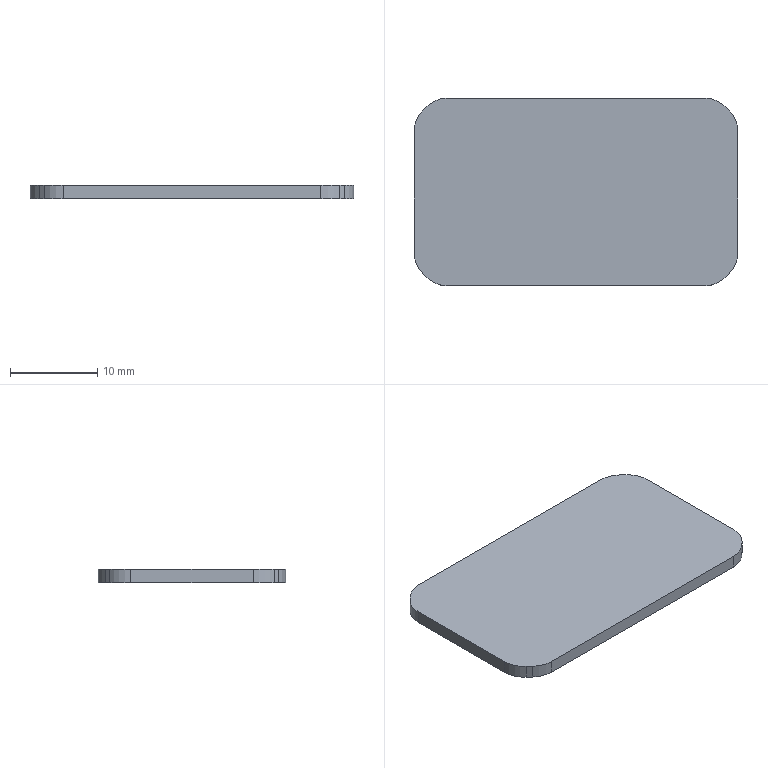Part | SolidWorks | features BaseBody 1 | 1 solid | 18 faces | box 37.1 x 21.5 x 1.5 mm | volume 1176 mm3 | plane 10 | cylinder 8 | commonest cylinder face diameters 6.5 x8
STEP:
#1=CARTESIAN_POINT('',(-18.55,7.,1.5));
#2=VERTEX_POINT('',#1);
#3=CARTESIAN_POINT('',(-18.55,-7.,1.5));
#4=VERTEX_POINT('',#3);
#5=CARTESIAN_POINT('',(-18.55,7.,1.5));
#6=DIRECTION('',(0.,-1.,0.));
#7=VECTOR('',#6,1000.);
#8=LINE('',#5,#7);
#9=EDGE_CURVE('',#2,#4,#8,.T.);
#10=ORIENTED_EDGE('',*,*,#9,.T.);
#11=CARTESIAN_POINT('',(-17.486,-9.405,1.5));
#12=VERTEX_POINT('',#11);
#13=CARTESIAN_POINT('',(-15.3,-7.,1.5));
#14=DIRECTION('',(0.,0.,1.));
#15=DIRECTION('',(-1.,0.,0.));
#16=AXIS2_PLACEMENT_3D('',#13,#14,#15);
#17=CIRCLE('',#16,3.25);
#18=EDGE_CURVE('',#4,#12,#17,.T.);
#19=ORIENTED_EDGE('',*,*,#18,.T.);
#20=CARTESIAN_POINT('',(-16.936,-9.905,1.5));
#21=VERTEX_POINT('',#20);
#22=CARTESIAN_POINT('',(-17.486,-9.405,1.5));
#23=DIRECTION('',(0.7399,-0.6727,0.));
#24=VECTOR('',#23,1000.);
#25=LINE('',#22,#24);
#26=EDGE_CURVE('',#12,#21,#25,.T.);
#27=ORIENTED_EDGE('',*,*,#26,.T.);
#28=CARTESIAN_POINT('',(-14.75,-10.75,1.5));
#29=VERTEX_POINT('',#28);
#30=CARTESIAN_POINT('',(-14.75,-7.5,1.5));
#31=DIRECTION('',(0.,0.,1.));
#32=DIRECTION('',(-0.6727,-0.7399,0.));
#33=AXIS2_PLACEMENT_3D('',#30,#31,#32);
#34=CIRCLE('',#33,3.25);
#35=EDGE_CURVE('',#21,#29,#34,.T.);
#36=ORIENTED_EDGE('',*,*,#35,.T.);
#37=CARTESIAN_POINT('',(14.75,-10.75,1.5));
#38=VERTEX_POINT('',#37);
#39=CARTESIAN_POINT('',(-14.75,-10.75,1.5));
#40=DIRECTION('',(1.,0.,0.));
#41=VECTOR('',#40,1000.);
#42=LINE('',#39,#41);
#43=EDGE_CURVE('',#29,#38,#42,.T.);
#44=ORIENTED_EDGE('',*,*,#43,.T.);
#45=CARTESIAN_POINT('',(16.936,-9.905,1.5));
#46=VERTEX_POINT('',#45);
#47=CARTESIAN_POINT('',(14.75,-7.5,1.5));
#48=DIRECTION('',(0.,0.,1.));
#49=DIRECTION('',(0.,-1.,0.));
#50=AXIS2_PLACEMENT_3D('',#47,#48,#49);
#51=CIRCLE('',#50,3.25);
#52=EDGE_CURVE('',#38,#46,#51,.T.);
#53=ORIENTED_EDGE('',*,*,#52,.T.);
#54=CARTESIAN_POINT('',(17.486,-9.405,1.5));
#55=VERTEX_POINT('',#54);
#56=CARTESIAN_POINT('',(16.936,-9.905,1.5));
#57=DIRECTION('',(0.7399,0.6727,0.));
#58=VECTOR('',#57,1000.);
#59=LINE('',#56,#58);
#60=EDGE_CURVE('',#46,#55,#59,.T.);
#61=ORIENTED_EDGE('',*,*,#60,.T.);
#62=CARTESIAN_POINT('',(18.55,-7.,1.5));
#63=VERTEX_POINT('',#62);
#64=CARTESIAN_POINT('',(15.3,-7.,1.5));
#65=DIRECTION('',(0.,0.,1.));
#66=DIRECTION('',(0.6727,-0.7399,0.));
#67=AXIS2_PLACEMENT_3D('',#64,#65,#66);
#68=CIRCLE('',#67,3.25);
#69=EDGE_CURVE('',#55,#63,#68,.T.);
#70=ORIENTED_EDGE('',*,*,#69,.T.);
#71=CARTESIAN_POINT('',(18.55,7.,1.5));
#72=VERTEX_POINT('',#71);
#73=CARTESIAN_POINT('',(18.55,-7.,1.5));
#74=DIRECTION('',(0.,1.,0.));
#75=VECTOR('',#74,1000.);
#76=LINE('',#73,#75);
#77=EDGE_CURVE('',#63,#72,#76,.T.);
#78=ORIENTED_EDGE('',*,*,#77,.T.);
#79=CARTESIAN_POINT('',(17.486,9.405,1.5));
#80=VERTEX_POINT('',#79);
#81=CARTESIAN_POINT('',(15.3,7.,1.5));
#82=DIRECTION('',(0.,0.,1.));
#83=DIRECTION('',(1.,0.,0.));
#84=AXIS2_PLACEMENT_3D('',#81,#82,#83);
#85=CIRCLE('',#84,3.25);
#86=EDGE_CURVE('',#72,#80,#85,.T.);
#87=ORIENTED_EDGE('',*,*,#86,.T.);
#88=CARTESIAN_POINT('',(16.936,9.905,1.5));
#89=VERTEX_POINT('',#88);
#90=CARTESIAN_POINT('',(17.486,9.405,1.5));
#91=DIRECTION('',(-0.7399,0.6727,0.));
#92=VECTOR('',#91,1000.);
#93=LINE('',#90,#92);
#94=EDGE_CURVE('',#80,#89,#93,.T.);
#95=ORIENTED_EDGE('',*,*,#94,.T.);
#96=CARTESIAN_POINT('',(14.75,10.75,1.5));
#97=VERTEX_POINT('',#96);
#98=CARTESIAN_POINT('',(14.75,7.5,1.5));
#99=DIRECTION('',(0.,0.,1.));
#100=DIRECTION('',(0.6727,0.7399,0.));
#101=AXIS2_PLACEMENT_3D('',#98,#99,#100);
#102=CIRCLE('',#101,3.25);
#103=EDGE_CURVE('',#89,#97,#102,.T.);
#104=ORIENTED_EDGE('',*,*,#103,.T.);
#105=CARTESIAN_POINT('',(-14.75,10.75,1.5));
#106=VERTEX_POINT('',#105);
#107=CARTESIAN_POINT('',(14.75,10.75,1.5));
#108=DIRECTION('',(-1.,0.,0.));
#109=VECTOR('',#108,1000.);
#110=LINE('',#107,#109);
#111=EDGE_CURVE('',#97,#106,#110,.T.);
#112=ORIENTED_EDGE('',*,*,#111,.T.);
#113=CARTESIAN_POINT('',(-16.936,9.905,1.5));
#114=VERTEX_POINT('',#113);
#115=CARTESIAN_POINT('',(-14.75,7.5,1.5));
#116=DIRECTION('',(0.,0.,1.));
#117=DIRECTION('',(0.,1.,0.));
#118=AXIS2_PLACEMENT_3D('',#115,#116,#117);
#119=CIRCLE('',#118,3.25);
#120=EDGE_CURVE('',#106,#114,#119,.T.);
#121=ORIENTED_EDGE('',*,*,#120,.T.);
#122=CARTESIAN_POINT('',(-17.486,9.405,1.5));
#123=VERTEX_POINT('',#122);
#124=CARTESIAN_POINT('',(-16.936,9.905,1.5));
#125=DIRECTION('',(-0.7399,-0.6727,0.));
#126=VECTOR('',#125,1000.);
#127=LINE('',#124,#126);
#128=EDGE_CURVE('',#114,#123,#127,.T.);
#129=ORIENTED_EDGE('',*,*,#128,.T.);
#130=CARTESIAN_POINT('',(-15.3,7.,1.5));
#131=DIRECTION('',(0.,0.,1.));
#132=DIRECTION('',(-0.6727,0.7399,0.));
#133=AXIS2_PLACEMENT_3D('',#130,#131,#132);
#134=CIRCLE('',#133,3.25);
#135=EDGE_CURVE('',#123,#2,#134,.T.);
#136=ORIENTED_EDGE('',*,*,#135,.T.);
#137=EDGE_LOOP('',(#10,#19,#27,#36,#44,#53,#61,#70,#78,#87,#95,#104,#112,#121,#129,#136));
#138=FACE_OUTER_BOUND('',#137,.T.);
#139=CARTESIAN_POINT('',(0.,0.,1.5));
#140=DIRECTION('',(0.,0.,1.));
#141=DIRECTION('',(1.,0.,0.));
#142=AXIS2_PLACEMENT_3D('',#139,#140,#141);
#143=PLANE('',#142);
#144=ADVANCED_FACE('',(#138),#143,.T.);
#145=CARTESIAN_POINT('',(-18.55,-7.,0.));
#146=VERTEX_POINT('',#145);
#147=CARTESIAN_POINT('',(-18.55,-7.,0.));
#148=DIRECTION('',(0.,0.,1.));
#149=VECTOR('',#148,1000.);
#150=LINE('',#147,#149);
#151=EDGE_CURVE('',#146,#4,#150,.T.);
#152=ORIENTED_EDGE('',*,*,#151,.T.);
#153=ORIENTED_EDGE('',*,*,#9,.F.);
#154=CARTESIAN_POINT('',(-18.55,7.,0.));
#155=VERTEX_POINT('',#154);
#156=CARTESIAN_POINT('',(-18.55,7.,0.));
#157=DIRECTION('',(0.,0.,1.));
#158=VECTOR('',#157,1000.);
#159=LINE('',#156,#158);
#160=EDGE_CURVE('',#155,#2,#159,.T.);
#161=ORIENTED_EDGE('',*,*,#160,.F.);
#162=CARTESIAN_POINT('',(-18.55,7.,0.));
#163=DIRECTION('',(0.,-1.,0.));
#164=VECTOR('',#163,1000.);
#165=LINE('',#162,#164);
#166=EDGE_CURVE('',#155,#146,#165,.T.);
#167=ORIENTED_EDGE('',*,*,#166,.T.);
#168=EDGE_LOOP('',(#152,#153,#161,#167));
#169=FACE_OUTER_BOUND('',#168,.T.);
#170=CARTESIAN_POINT('',(-18.55,7.,0.));
#171=DIRECTION('',(-1.,0.,0.));
#172=DIRECTION('',(0.,0.,1.));
#173=AXIS2_PLACEMENT_3D('',#170,#171,#172);
#174=PLANE('',#173);
#175=ADVANCED_FACE('',(#169),#174,.T.);
#176=CARTESIAN_POINT('',(-17.486,-9.405,0.));
#177=VERTEX_POINT('',#176);
#178=CARTESIAN_POINT('',(-17.486,-9.405,0.));
#179=DIRECTION('',(0.,0.,1.));
#180=VECTOR('',#179,1000.);
#181=LINE('',#178,#180);
#182=EDGE_CURVE('',#177,#12,#181,.T.);
#183=ORIENTED_EDGE('',*,*,#182,.T.);
#184=ORIENTED_EDGE('',*,*,#18,.F.);
#185=ORIENTED_EDGE('',*,*,#151,.F.);
#186=CARTESIAN_POINT('',(-15.3,-7.,0.));
#187=DIRECTION('',(0.,0.,1.));
#188=DIRECTION('',(-1.,0.,0.));
#189=AXIS2_PLACEMENT_3D('',#186,#187,#188);
#190=CIRCLE('',#189,3.25);
#191=EDGE_CURVE('',#146,#177,#190,.T.);
#192=ORIENTED_EDGE('',*,*,#191,.T.);
#193=EDGE_LOOP('',(#183,#184,#185,#192));
#194=FACE_OUTER_BOUND('',#193,.T.);
#195=CARTESIAN_POINT('',(-15.3,-7.,0.));
#196=DIRECTION('',(0.,0.,1.));
#197=DIRECTION('',(1.,0.,0.));
#198=AXIS2_PLACEMENT_3D('',#195,#196,#197);
#199=CYLINDRICAL_SURFACE('',#198,3.25);
#200=ADVANCED_FACE('',(#194),#199,.T.);
#201=CARTESIAN_POINT('',(-16.936,-9.905,0.));
#202=VERTEX_POINT('',#201);
#203=CARTESIAN_POINT('',(-16.936,-9.905,0.));
#204=DIRECTION('',(0.,0.,1.));
#205=VECTOR('',#204,1000.);
#206=LINE('',#203,#205);
#207=EDGE_CURVE('',#202,#21,#206,.T.);
#208=ORIENTED_EDGE('',*,*,#207,.T.);
#209=ORIENTED_EDGE('',*,*,#26,.F.);
#210=ORIENTED_EDGE('',*,*,#182,.F.);
#211=CARTESIAN_POINT('',(-17.486,-9.405,0.));
#212=DIRECTION('',(0.7399,-0.6727,0.));
#213=VECTOR('',#212,1000.);
#214=LINE('',#211,#213);
#215=EDGE_CURVE('',#177,#202,#214,.T.);
#216=ORIENTED_EDGE('',*,*,#215,.T.);
#217=EDGE_LOOP('',(#208,#209,#210,#216));
#218=FACE_OUTER_BOUND('',#217,.T.);
#219=CARTESIAN_POINT('',(-17.486,-9.405,0.));
#220=DIRECTION('',(-0.6727,-0.7399,0.));
#221=DIRECTION('',(-0.7399,0.6727,0.));
#222=AXIS2_PLACEMENT_3D('',#219,#220,#221);
#223=PLANE('',#222);
#224=ADVANCED_FACE('',(#218),#223,.T.);
#225=CARTESIAN_POINT('',(-14.75,-10.75,0.));
#226=VERTEX_POINT('',#225);
#227=CARTESIAN_POINT('',(-14.75,-10.75,0.));
#228=DIRECTION('',(0.,0.,1.));
#229=VECTOR('',#228,1000.);
#230=LINE('',#227,#229);
#231=EDGE_CURVE('',#226,#29,#230,.T.);
#232=ORIENTED_EDGE('',*,*,#231,.T.);
#233=ORIENTED_EDGE('',*,*,#35,.F.);
#234=ORIENTED_EDGE('',*,*,#207,.F.);
#235=CARTESIAN_POINT('',(-14.75,-7.5,0.));
#236=DIRECTION('',(0.,0.,1.));
#237=DIRECTION('',(-0.6727,-0.7399,0.));
#238=AXIS2_PLACEMENT_3D('',#235,#236,#237);
#239=CIRCLE('',#238,3.25);
#240=EDGE_CURVE('',#202,#226,#239,.T.);
#241=ORIENTED_EDGE('',*,*,#240,.T.);
#242=EDGE_LOOP('',(#232,#233,#234,#241));
#243=FACE_OUTER_BOUND('',#242,.T.);
#244=CARTESIAN_POINT('',(-14.75,-7.5,0.));
#245=DIRECTION('',(0.,0.,1.));
#246=DIRECTION('',(1.,0.,0.));
#247=AXIS2_PLACEMENT_3D('',#244,#245,#246);
#248=CYLINDRICAL_SURFACE('',#247,3.25);
#249=ADVANCED_FACE('',(#243),#248,.T.);
#250=CARTESIAN_POINT('',(14.75,-10.75,0.));
#251=VERTEX_POINT('',#250);
#252=CARTESIAN_POINT('',(14.75,-10.75,0.));
#253=DIRECTION('',(0.,0.,1.));
#254=VECTOR('',#253,1000.);
#255=LINE('',#252,#254);
#256=EDGE_CURVE('',#251,#38,#255,.T.);
#257=ORIENTED_EDGE('',*,*,#256,.T.);
#258=ORIENTED_EDGE('',*,*,#43,.F.);
#259=ORIENTED_EDGE('',*,*,#231,.F.);
#260=CARTESIAN_POINT('',(-14.75,-10.75,0.));
#261=DIRECTION('',(1.,0.,0.));
#262=VECTOR('',#261,1000.);
#263=LINE('',#260,#262);
#264=EDGE_CURVE('',#226,#251,#263,.T.);
#265=ORIENTED_EDGE('',*,*,#264,.T.);
#266=EDGE_LOOP('',(#257,#258,#259,#265));
#267=FACE_OUTER_BOUND('',#266,.T.);
#268=CARTESIAN_POINT('',(-14.75,-10.75,0.));
#269=DIRECTION('',(0.,-1.,0.));
#270=DIRECTION('',(0.,0.,-1.));
#271=AXIS2_PLACEMENT_3D('',#268,#269,#270);
#272=PLANE('',#271);
#273=ADVANCED_FACE('',(#267),#272,.T.);
#274=CARTESIAN_POINT('',(16.936,-9.905,0.));
#275=VERTEX_POINT('',#274);
#276=CARTESIAN_POINT('',(16.936,-9.905,0.));
#277=DIRECTION('',(0.,0.,1.));
#278=VECTOR('',#277,1000.);
#279=LINE('',#276,#278);
#280=EDGE_CURVE('',#275,#46,#279,.T.);
#281=ORIENTED_EDGE('',*,*,#280,.T.);
#282=ORIENTED_EDGE('',*,*,#52,.F.);
#283=ORIENTED_EDGE('',*,*,#256,.F.);
#284=CARTESIAN_POINT('',(14.75,-7.5,0.));
#285=DIRECTION('',(0.,0.,1.));
#286=DIRECTION('',(0.,-1.,0.));
#287=AXIS2_PLACEMENT_3D('',#284,#285,#286);
#288=CIRCLE('',#287,3.25);
#289=EDGE_CURVE('',#251,#275,#288,.T.);
#290=ORIENTED_EDGE('',*,*,#289,.T.);
#291=EDGE_LOOP('',(#281,#282,#283,#290));
#292=FACE_OUTER_BOUND('',#291,.T.);
#293=CARTESIAN_POINT('',(14.75,-7.5,0.));
#294=DIRECTION('',(0.,0.,1.));
#295=DIRECTION('',(1.,0.,0.));
#296=AXIS2_PLACEMENT_3D('',#293,#294,#295);
#297=CYLINDRICAL_SURFACE('',#296,3.25);
#298=ADVANCED_FACE('',(#292),#297,.T.);
#299=CARTESIAN_POINT('',(17.486,-9.405,0.));
#300=VERTEX_POINT('',#299);
#301=CARTESIAN_POINT('',(17.486,-9.405,0.));
#302=DIRECTION('',(0.,0.,1.));
#303=VECTOR('',#302,1000.);
#304=LINE('',#301,#303);
#305=EDGE_CURVE('',#300,#55,#304,.T.);
#306=ORIENTED_EDGE('',*,*,#305,.T.);
#307=ORIENTED_EDGE('',*,*,#60,.F.);
#308=ORIENTED_EDGE('',*,*,#280,.F.);
#309=CARTESIAN_POINT('',(16.936,-9.905,0.));
#310=DIRECTION('',(0.7399,0.6727,0.));
#311=VECTOR('',#310,1000.);
#312=LINE('',#309,#311);
#313=EDGE_CURVE('',#275,#300,#312,.T.);
#314=ORIENTED_EDGE('',*,*,#313,.T.);
#315=EDGE_LOOP('',(#306,#307,#308,#314));
#316=FACE_OUTER_BOUND('',#315,.T.);
#317=CARTESIAN_POINT('',(16.936,-9.905,0.));
#318=DIRECTION('',(0.6727,-0.7399,0.));
#319=DIRECTION('',(0.,0.,-1.));
#320=AXIS2_PLACEMENT_3D('',#317,#318,#319);
#321=PLANE('',#320);
#322=ADVANCED_FACE('',(#316),#321,.T.);
#323=CARTESIAN_POINT('',(18.55,-7.,0.));
#324=VERTEX_POINT('',#323);
#325=CARTESIAN_POINT('',(18.55,-7.,0.));
#326=DIRECTION('',(0.,0.,1.));
#327=VECTOR('',#326,1000.);
#328=LINE('',#325,#327);
#329=EDGE_CURVE('',#324,#63,#328,.T.);
#330=ORIENTED_EDGE('',*,*,#329,.T.);
#331=ORIENTED_EDGE('',*,*,#69,.F.);
#332=ORIENTED_EDGE('',*,*,#305,.F.);
#333=CARTESIAN_POINT('',(15.3,-7.,0.));
#334=DIRECTION('',(0.,0.,1.));
#335=DIRECTION('',(0.6727,-0.7399,0.));
#336=AXIS2_PLACEMENT_3D('',#333,#334,#335);
#337=CIRCLE('',#336,3.25);
#338=EDGE_CURVE('',#300,#324,#337,.T.);
#339=ORIENTED_EDGE('',*,*,#338,.T.);
#340=EDGE_LOOP('',(#330,#331,#332,#339));
#341=FACE_OUTER_BOUND('',#340,.T.);
#342=CARTESIAN_POINT('',(15.3,-7.,0.));
#343=DIRECTION('',(0.,0.,1.));
#344=DIRECTION('',(1.,0.,0.));
#345=AXIS2_PLACEMENT_3D('',#342,#343,#344);
#346=CYLINDRICAL_SURFACE('',#345,3.25);
#347=ADVANCED_FACE('',(#341),#346,.T.);
#348=CARTESIAN_POINT('',(18.55,7.,0.));
#349=VERTEX_POINT('',#348);
#350=CARTESIAN_POINT('',(18.55,7.,0.));
#351=DIRECTION('',(0.,0.,1.));
#352=VECTOR('',#351,1000.);
#353=LINE('',#350,#352);
#354=EDGE_CURVE('',#349,#72,#353,.T.);
#355=ORIENTED_EDGE('',*,*,#354,.T.);
#356=ORIENTED_EDGE('',*,*,#77,.F.);
#357=ORIENTED_EDGE('',*,*,#329,.F.);
#358=CARTESIAN_POINT('',(18.55,-7.,0.));
#359=DIRECTION('',(0.,1.,0.));
#360=VECTOR('',#359,1000.);
#361=LINE('',#358,#360);
#362=EDGE_CURVE('',#324,#349,#361,.T.);
#363=ORIENTED_EDGE('',*,*,#362,.T.);
#364=EDGE_LOOP('',(#355,#356,#357,#363));
#365=FACE_OUTER_BOUND('',#364,.T.);
#366=CARTESIAN_POINT('',(18.55,-7.,0.));
#367=DIRECTION('',(1.,0.,0.));
#368=DIRECTION('',(0.,1.,0.));
#369=AXIS2_PLACEMENT_3D('',#366,#367,#368);
#370=PLANE('',#369);
#371=ADVANCED_FACE('',(#365),#370,.T.);
#372=CARTESIAN_POINT('',(17.486,9.405,0.));
#373=VERTEX_POINT('',#372);
#374=CARTESIAN_POINT('',(17.486,9.405,0.));
#375=DIRECTION('',(0.,0.,1.));
#376=VECTOR('',#375,1000.);
#377=LINE('',#374,#376);
#378=EDGE_CURVE('',#373,#80,#377,.T.);
#379=ORIENTED_EDGE('',*,*,#378,.T.);
#380=ORIENTED_EDGE('',*,*,#86,.F.);
#381=ORIENTED_EDGE('',*,*,#354,.F.);
#382=CARTESIAN_POINT('',(15.3,7.,0.));
#383=DIRECTION('',(0.,0.,1.));
#384=DIRECTION('',(1.,0.,0.));
#385=AXIS2_PLACEMENT_3D('',#382,#383,#384);
#386=CIRCLE('',#385,3.25);
#387=EDGE_CURVE('',#349,#373,#386,.T.);
#388=ORIENTED_EDGE('',*,*,#387,.T.);
#389=EDGE_LOOP('',(#379,#380,#381,#388));
#390=FACE_OUTER_BOUND('',#389,.T.);
#391=CARTESIAN_POINT('',(15.3,7.,0.));
#392=DIRECTION('',(0.,0.,1.));
#393=DIRECTION('',(1.,0.,0.));
#394=AXIS2_PLACEMENT_3D('',#391,#392,#393);
#395=CYLINDRICAL_SURFACE('',#394,3.25);
#396=ADVANCED_FACE('',(#390),#395,.T.);
#397=CARTESIAN_POINT('',(16.936,9.905,0.));
#398=VERTEX_POINT('',#397);
#399=CARTESIAN_POINT('',(16.936,9.905,0.));
#400=DIRECTION('',(0.,0.,1.));
#401=VECTOR('',#400,1000.);
#402=LINE('',#399,#401);
#403=EDGE_CURVE('',#398,#89,#402,.T.);
#404=ORIENTED_EDGE('',*,*,#403,.T.);
#405=ORIENTED_EDGE('',*,*,#94,.F.);
#406=ORIENTED_EDGE('',*,*,#378,.F.);
#407=CARTESIAN_POINT('',(17.486,9.405,0.));
#408=DIRECTION('',(-0.7399,0.6727,0.));
#409=VECTOR('',#408,1000.);
#410=LINE('',#407,#409);
#411=EDGE_CURVE('',#373,#398,#410,.T.);
#412=ORIENTED_EDGE('',*,*,#411,.T.);
#413=EDGE_LOOP('',(#404,#405,#406,#412));
#414=FACE_OUTER_BOUND('',#413,.T.);
#415=CARTESIAN_POINT('',(17.486,9.405,0.));
#416=DIRECTION('',(0.6727,0.7399,0.));
#417=DIRECTION('',(0.,0.,-1.));
#418=AXIS2_PLACEMENT_3D('',#415,#416,#417);
#419=PLANE('',#418);
#420=ADVANCED_FACE('',(#414),#419,.T.);
#421=CARTESIAN_POINT('',(14.75,10.75,0.));
#422=VERTEX_POINT('',#421);
#423=CARTESIAN_POINT('',(14.75,10.75,0.));
#424=DIRECTION('',(0.,0.,1.));
#425=VECTOR('',#424,1000.);
#426=LINE('',#423,#425);
#427=EDGE_CURVE('',#422,#97,#426,.T.);
#428=ORIENTED_EDGE('',*,*,#427,.T.);
#429=ORIENTED_EDGE('',*,*,#103,.F.);
#430=ORIENTED_EDGE('',*,*,#403,.F.);
#431=CARTESIAN_POINT('',(14.75,7.5,0.));
#432=DIRECTION('',(0.,0.,1.));
#433=DIRECTION('',(0.6727,0.7399,0.));
#434=AXIS2_PLACEMENT_3D('',#431,#432,#433);
#435=CIRCLE('',#434,3.25);
#436=EDGE_CURVE('',#398,#422,#435,.T.);
#437=ORIENTED_EDGE('',*,*,#436,.T.);
#438=EDGE_LOOP('',(#428,#429,#430,#437));
#439=FACE_OUTER_BOUND('',#438,.T.);
#440=CARTESIAN_POINT('',(14.75,7.5,0.));
#441=DIRECTION('',(0.,0.,1.));
#442=DIRECTION('',(1.,0.,0.));
#443=AXIS2_PLACEMENT_3D('',#440,#441,#442);
#444=CYLINDRICAL_SURFACE('',#443,3.25);
#445=ADVANCED_FACE('',(#439),#444,.T.);
#446=CARTESIAN_POINT('',(-14.75,10.75,0.));
#447=VERTEX_POINT('',#446);
#448=CARTESIAN_POINT('',(-14.75,10.75,0.));
#449=DIRECTION('',(0.,0.,1.));
#450=VECTOR('',#449,1000.);
#451=LINE('',#448,#450);
#452=EDGE_CURVE('',#447,#106,#451,.T.);
#453=ORIENTED_EDGE('',*,*,#452,.T.);
#454=ORIENTED_EDGE('',*,*,#111,.F.);
#455=ORIENTED_EDGE('',*,*,#427,.F.);
#456=CARTESIAN_POINT('',(14.75,10.75,0.));
#457=DIRECTION('',(-1.,0.,0.));
#458=VECTOR('',#457,1000.);
#459=LINE('',#456,#458);
#460=EDGE_CURVE('',#422,#447,#459,.T.);
#461=ORIENTED_EDGE('',*,*,#460,.T.);
#462=EDGE_LOOP('',(#453,#454,#455,#461));
#463=FACE_OUTER_BOUND('',#462,.T.);
#464=CARTESIAN_POINT('',(14.75,10.75,0.));
#465=DIRECTION('',(0.,1.,0.));
#466=DIRECTION('',(1.,0.,0.));
#467=AXIS2_PLACEMENT_3D('',#464,#465,#466);
#468=PLANE('',#467);
#469=ADVANCED_FACE('',(#463),#468,.T.);
#470=CARTESIAN_POINT('',(-16.936,9.905,0.));
#471=VERTEX_POINT('',#470);
#472=CARTESIAN_POINT('',(-16.936,9.905,0.));
#473=DIRECTION('',(0.,0.,1.));
#474=VECTOR('',#473,1000.);
#475=LINE('',#472,#474);
#476=EDGE_CURVE('',#471,#114,#475,.T.);
#477=ORIENTED_EDGE('',*,*,#476,.T.);
#478=ORIENTED_EDGE('',*,*,#120,.F.);
#479=ORIENTED_EDGE('',*,*,#452,.F.);
#480=CARTESIAN_POINT('',(-14.75,7.5,0.));
#481=DIRECTION('',(0.,0.,1.));
#482=DIRECTION('',(0.,1.,0.));
#483=AXIS2_PLACEMENT_3D('',#480,#481,#482);
#484=CIRCLE('',#483,3.25);
#485=EDGE_CURVE('',#447,#471,#484,.T.);
#486=ORIENTED_EDGE('',*,*,#485,.T.);
#487=EDGE_LOOP('',(#477,#478,#479,#486));
#488=FACE_OUTER_BOUND('',#487,.T.);
#489=CARTESIAN_POINT('',(-14.75,7.5,0.));
#490=DIRECTION('',(0.,0.,1.));
#491=DIRECTION('',(1.,0.,0.));
#492=AXIS2_PLACEMENT_3D('',#489,#490,#491);
#493=CYLINDRICAL_SURFACE('',#492,3.25);
#494=ADVANCED_FACE('',(#488),#493,.T.);
#495=CARTESIAN_POINT('',(-17.486,9.405,0.));
#496=VERTEX_POINT('',#495);
#497=CARTESIAN_POINT('',(-17.486,9.405,0.));
#498=DIRECTION('',(0.,0.,1.));
#499=VECTOR('',#498,1000.);
#500=LINE('',#497,#499);
#501=EDGE_CURVE('',#496,#123,#500,.T.);
#502=ORIENTED_EDGE('',*,*,#501,.T.);
#503=ORIENTED_EDGE('',*,*,#128,.F.);
#504=ORIENTED_EDGE('',*,*,#476,.F.);
#505=CARTESIAN_POINT('',(-16.936,9.905,0.));
#506=DIRECTION('',(-0.7399,-0.6727,0.));
#507=VECTOR('',#506,1000.);
#508=LINE('',#505,#507);
#509=EDGE_CURVE('',#471,#496,#508,.T.);
#510=ORIENTED_EDGE('',*,*,#509,.T.);
#511=EDGE_LOOP('',(#502,#503,#504,#510));
#512=FACE_OUTER_BOUND('',#511,.T.);
#513=CARTESIAN_POINT('',(-16.936,9.905,0.));
#514=DIRECTION('',(-0.6727,0.7399,0.));
#515=DIRECTION('',(0.,0.,1.));
#516=AXIS2_PLACEMENT_3D('',#513,#514,#515);
#517=PLANE('',#516);
#518=ADVANCED_FACE('',(#512),#517,.T.);
#519=ORIENTED_EDGE('',*,*,#160,.T.);
#520=ORIENTED_EDGE('',*,*,#135,.F.);
#521=ORIENTED_EDGE('',*,*,#501,.F.);
#522=CARTESIAN_POINT('',(-15.3,7.,0.));
#523=DIRECTION('',(0.,0.,1.));
#524=DIRECTION('',(-0.6727,0.7399,0.));
#525=AXIS2_PLACEMENT_3D('',#522,#523,#524);
#526=CIRCLE('',#525,3.25);
#527=EDGE_CURVE('',#496,#155,#526,.T.);
#528=ORIENTED_EDGE('',*,*,#527,.T.);
#529=EDGE_LOOP('',(#519,#520,#521,#528));
#530=FACE_OUTER_BOUND('',#529,.T.);
#531=CARTESIAN_POINT('',(-15.3,7.,0.));
#532=DIRECTION('',(0.,0.,1.));
#533=DIRECTION('',(1.,0.,0.));
#534=AXIS2_PLACEMENT_3D('',#531,#532,#533);
#535=CYLINDRICAL_SURFACE('',#534,3.25);
#536=ADVANCED_FACE('',(#530),#535,.T.);
#537=ORIENTED_EDGE('',*,*,#509,.F.);
#538=ORIENTED_EDGE('',*,*,#485,.F.);
#539=ORIENTED_EDGE('',*,*,#460,.F.);
#540=ORIENTED_EDGE('',*,*,#436,.F.);
#541=ORIENTED_EDGE('',*,*,#411,.F.);
#542=ORIENTED_EDGE('',*,*,#387,.F.);
#543=ORIENTED_EDGE('',*,*,#362,.F.);
#544=ORIENTED_EDGE('',*,*,#338,.F.);
#545=ORIENTED_EDGE('',*,*,#313,.F.);
#546=ORIENTED_EDGE('',*,*,#289,.F.);
#547=ORIENTED_EDGE('',*,*,#264,.F.);
#548=ORIENTED_EDGE('',*,*,#240,.F.);
#549=ORIENTED_EDGE('',*,*,#215,.F.);
#550=ORIENTED_EDGE('',*,*,#191,.F.);
#551=ORIENTED_EDGE('',*,*,#166,.F.);
#552=ORIENTED_EDGE('',*,*,#527,.F.);
#553=EDGE_LOOP('',(#537,#538,#539,#540,#541,#542,#543,#544,#545,#546,#547,#548,#549,#550,#551,#552));
#554=FACE_OUTER_BOUND('',#553,.T.);
#555=CARTESIAN_POINT('',(0.,0.,0.));
#556=DIRECTION('',(0.,0.,1.));
#557=DIRECTION('',(1.,0.,0.));
#558=AXIS2_PLACEMENT_3D('',#555,#556,#557);
#559=PLANE('',#558);
#560=ADVANCED_FACE('',(#554),#559,.F.);
#561=CLOSED_SHELL('',(#144,#175,#200,#224,#249,#273,#298,#322,#347,#371,#396,#420,#445,#469,#494,#518,#536,#560));
#562=MANIFOLD_SOLID_BREP('',#561);
#563=CARTESIAN_POINT('',(0.,0.,0.));
#564=DIRECTION('',(0.,0.,1.));
#565=DIRECTION('',(1.,0.,0.));
#566=AXIS2_PLACEMENT_3D('',#563,#564,#565);
#567=(LENGTH_UNIT()NAMED_UNIT(*)SI_UNIT(.MILLI.,.METRE.));
#568=UNCERTAINTY_MEASURE_WITH_UNIT(LENGTH_MEASURE(0.00001),#567,'','');
#569=(NAMED_UNIT(*)PLANE_ANGLE_UNIT()SI_UNIT($,.RADIAN.));
#570=(NAMED_UNIT(*)SI_UNIT($,.STERADIAN.)SOLID_ANGLE_UNIT());
#571=(GEOMETRIC_REPRESENTATION_CONTEXT(3)GLOBAL_UNCERTAINTY_ASSIGNED_CONTEXT((#568))GLOBAL_UNIT_ASSIGNED_CONTEXT((#567,#569,#570))REPRESENTATION_CONTEXT('',''));
#572=ADVANCED_BREP_SHAPE_REPRESENTATION('',(#562,#566),#571);